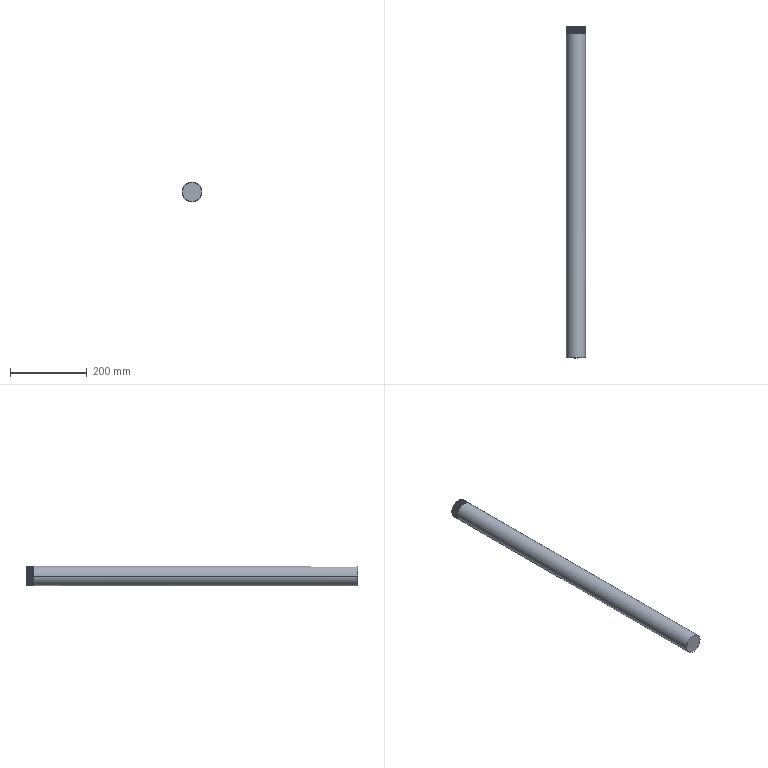Part | STEP file | Input 1-1 | 1 solid | 48 faces | box 50 x 866.727 x 50 mm | volume 1701788 mm3 | cylinder 42 | plane 3 | spline 3 | commonest cylinder face diameters 50 x42